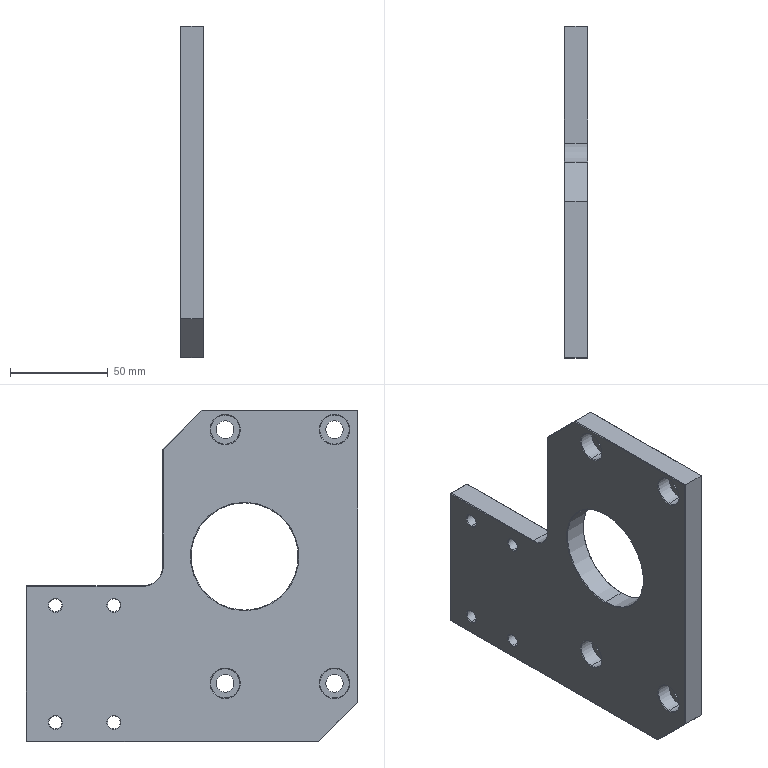Part | STEP file | PN_0001 motor fixing plate_Default | 1 solid | 113 faces | box 12 x 170 x 170 mm | volume 228176 mm3 | plane 40 | cone 38 | cylinder 35 | commonest cylinder face diameters 6.6 x8 9 x8 11 x8 15 x8 55 x2 20 x1